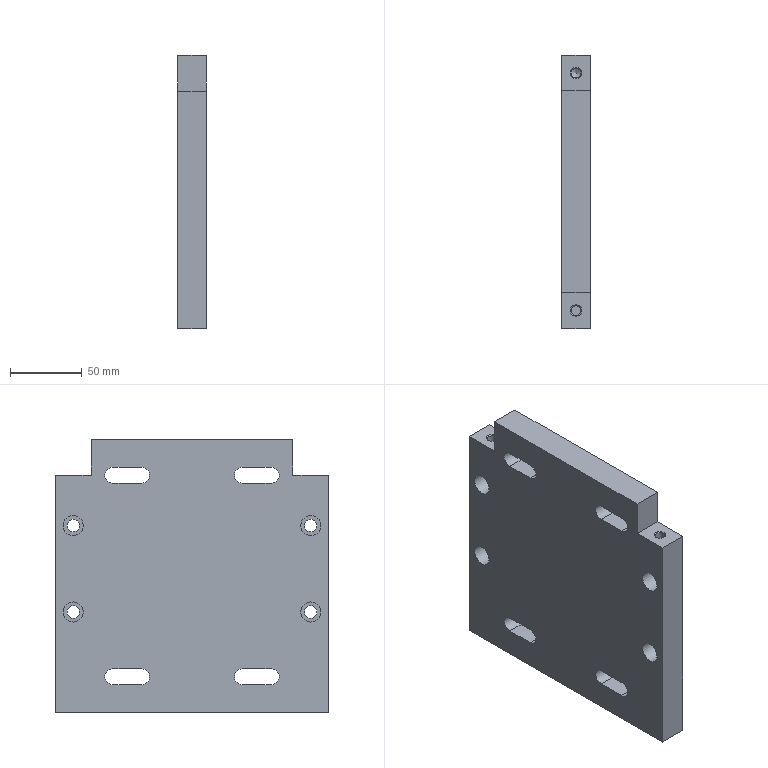Part | STEP file | YBQDJ-FLJ-5 | 1 solid | 44 faces | box 20 x 190 x 190 mm | volume 661776 mm3 | plane 23 | cylinder 18 | cone 3 | commonest cylinder face diameters 11 x8 8.7 x4 14 x4 6.8 x2